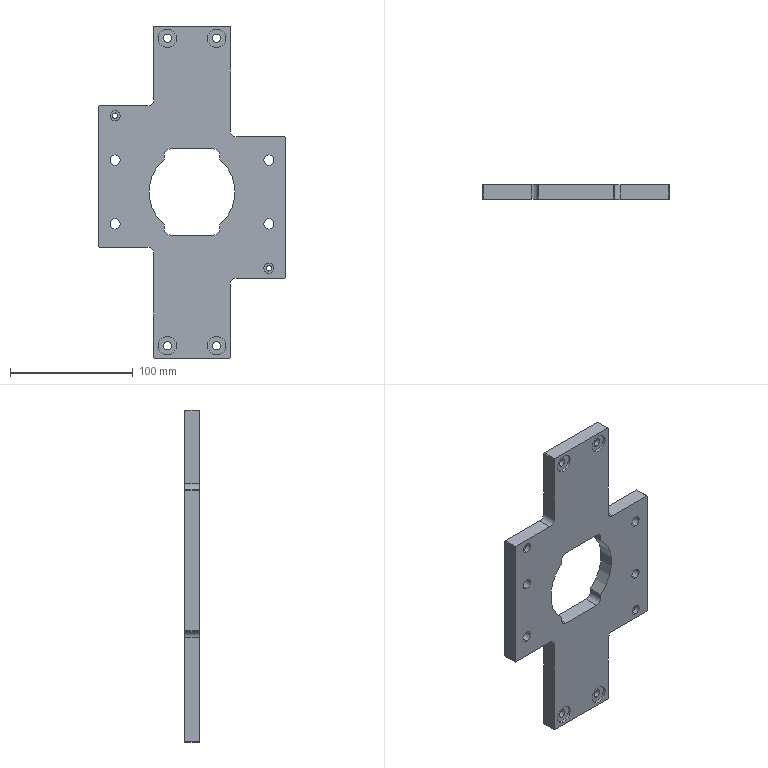Part | SolidWorks | features ICE 6, HoleWzd 3, Chamfer 1, Extrusion 1, Fillet 1 | 1 solid | 106 faces | box 152 x 12 x 270 mm | volume 265113 mm3 | cylinder 62 | plane 44 | commonest cylinder face diameters 6.6 x8 8.4 x8 10 x8 11 x8 15 x8 16.1 x8